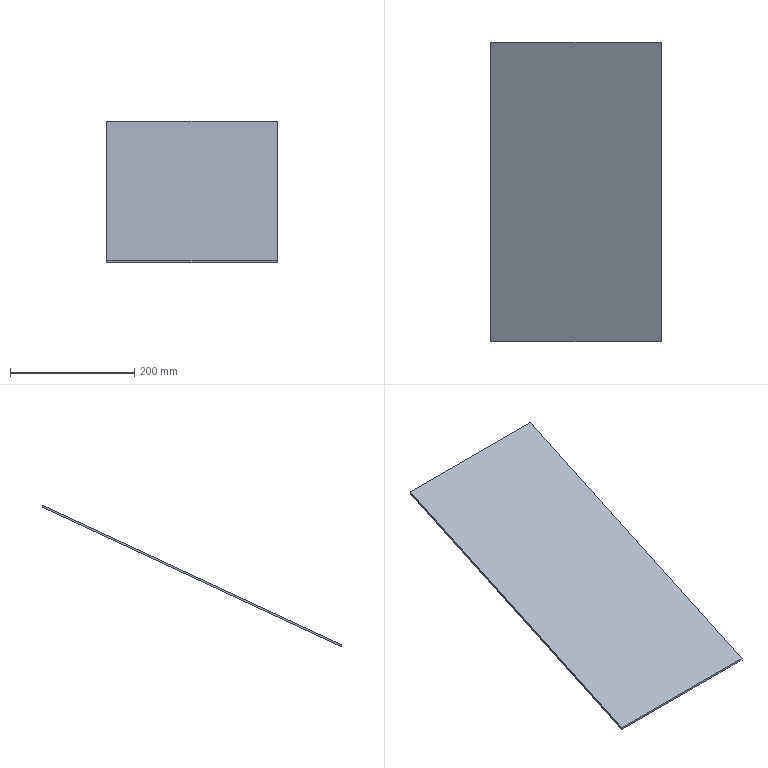Part | NX | features solid 2 | 1 solid | 6 faces | box 274 x 482 x 228.07 mm | volume 437163 mm3 | plane 6
STEP:
#1=CARTESIAN_POINT('',(-137.,22.,-157.195));
#2=VERTEX_POINT('',#1);
#3=CARTESIAN_POINT('',(-137.,22.,-160.505));
#4=VERTEX_POINT('',#3);
#5=CARTESIAN_POINT('',(-137.,22.,-497.5));
#6=DIRECTION('',(0.,0.,-1.));
#7=VECTOR('',#6,1000.);
#8=LINE('',#5,#7);
#9=EDGE_CURVE('',#2,#4,#8,.T.);
#10=ORIENTED_EDGE('',*,*,#9,.T.);
#11=CARTESIAN_POINT('',(-137.,-460.,-385.266));
#12=VERTEX_POINT('',#11);
#13=CARTESIAN_POINT('',(-137.,-98.862,-216.864));
#14=DIRECTION('',(0.,-0.9063,-0.4226));
#15=VECTOR('',#14,1000.);
#16=LINE('',#13,#15);
#17=EDGE_CURVE('',#4,#12,#16,.T.);
#18=ORIENTED_EDGE('',*,*,#17,.T.);
#19=CARTESIAN_POINT('',(-137.,-460.,-381.956));
#20=VERTEX_POINT('',#19);
#21=CARTESIAN_POINT('',(-137.,-460.,-97.5));
#22=DIRECTION('',(0.,0.,1.));
#23=VECTOR('',#22,1000.);
#24=LINE('',#21,#23);
#25=EDGE_CURVE('',#20,#12,#24,.F.);
#26=ORIENTED_EDGE('',*,*,#25,.F.);
#27=CARTESIAN_POINT('',(-137.,-100.13,-214.146));
#28=DIRECTION('',(0.,-0.9063,-0.4226));
#29=VECTOR('',#28,1000.);
#30=LINE('',#27,#29);
#31=EDGE_CURVE('',#2,#20,#30,.T.);
#32=ORIENTED_EDGE('',*,*,#31,.F.);
#33=EDGE_LOOP('',(#10,#18,#26,#32));
#34=FACE_BOUND('',#33,.T.);
#35=CARTESIAN_POINT('',(-137.,32.,-497.5));
#36=DIRECTION('',(1.,0.,0.));
#37=DIRECTION('',(0.,0.,-1.));
#38=AXIS2_PLACEMENT_3D('',#35,#36,#37);
#39=PLANE('',#38);
#40=ADVANCED_FACE('',(#34),#39,.F.);
#41=ORIENTED_EDGE('',*,*,#25,.T.);
#42=CARTESIAN_POINT('',(137.,-460.,-385.266));
#43=VERTEX_POINT('',#42);
#44=CARTESIAN_POINT('',(1125.,-460.,-385.266));
#45=DIRECTION('',(-1.,0.,0.));
#46=VECTOR('',#45,1000.);
#47=LINE('',#44,#46);
#48=EDGE_CURVE('',#12,#43,#47,.F.);
#49=ORIENTED_EDGE('',*,*,#48,.T.);
#50=CARTESIAN_POINT('',(137.,-460.,-381.956));
#51=VERTEX_POINT('',#50);
#52=CARTESIAN_POINT('',(137.,-460.,-497.5));
#53=DIRECTION('',(0.,0.,1.));
#54=VECTOR('',#53,1000.);
#55=LINE('',#52,#54);
#56=EDGE_CURVE('',#51,#43,#55,.F.);
#57=ORIENTED_EDGE('',*,*,#56,.F.);
#58=CARTESIAN_POINT('',(1125.,-460.,-381.956));
#59=DIRECTION('',(-1.,0.,0.));
#60=VECTOR('',#59,1000.);
#61=LINE('',#58,#60);
#62=EDGE_CURVE('',#20,#51,#61,.F.);
#63=ORIENTED_EDGE('',*,*,#62,.F.);
#64=EDGE_LOOP('',(#41,#49,#57,#63));
#65=FACE_BOUND('',#64,.T.);
#66=CARTESIAN_POINT('',(1125.,-460.,-97.5));
#67=DIRECTION('',(0.,-1.,0.));
#68=DIRECTION('',(-1.,0.,0.));
#69=AXIS2_PLACEMENT_3D('',#66,#67,#68);
#70=PLANE('',#69);
#71=ADVANCED_FACE('',(#65),#70,.T.);
#72=ORIENTED_EDGE('',*,*,#56,.T.);
#73=CARTESIAN_POINT('',(137.,22.,-160.505));
#74=VERTEX_POINT('',#73);
#75=CARTESIAN_POINT('',(137.,7.,-167.5));
#76=DIRECTION('',(0.,-0.9063,-0.4226));
#77=VECTOR('',#76,1000.);
#78=LINE('',#75,#77);
#79=EDGE_CURVE('',#74,#43,#78,.T.);
#80=ORIENTED_EDGE('',*,*,#79,.F.);
#81=CARTESIAN_POINT('',(137.,22.,-157.195));
#82=VERTEX_POINT('',#81);
#83=CARTESIAN_POINT('',(137.,22.,26.231));
#84=DIRECTION('',(0.,0.,-1.));
#85=VECTOR('',#84,1000.);
#86=LINE('',#83,#85);
#87=EDGE_CURVE('',#82,#74,#86,.T.);
#88=ORIENTED_EDGE('',*,*,#87,.F.);
#89=CARTESIAN_POINT('',(137.,5.732,-164.781));
#90=DIRECTION('',(0.,-0.9063,-0.4226));
#91=VECTOR('',#90,1000.);
#92=LINE('',#89,#91);
#93=EDGE_CURVE('',#82,#51,#92,.T.);
#94=ORIENTED_EDGE('',*,*,#93,.T.);
#95=EDGE_LOOP('',(#72,#80,#88,#94));
#96=FACE_BOUND('',#95,.T.);
#97=CARTESIAN_POINT('',(137.,32.,-497.5));
#98=DIRECTION('',(-1.,0.,0.));
#99=DIRECTION('',(0.,0.,-1.));
#100=AXIS2_PLACEMENT_3D('',#97,#98,#99);
#101=PLANE('',#100);
#102=ADVANCED_FACE('',(#96),#101,.F.);
#103=CARTESIAN_POINT('',(-17.526,22.,-157.195));
#104=DIRECTION('',(1.,0.,0.));
#105=VECTOR('',#104,1000.);
#106=LINE('',#103,#105);
#107=EDGE_CURVE('',#2,#82,#106,.T.);
#108=ORIENTED_EDGE('',*,*,#107,.T.);
#109=ORIENTED_EDGE('',*,*,#87,.T.);
#110=CARTESIAN_POINT('',(-17.526,22.,-160.505));
#111=DIRECTION('',(1.,0.,0.));
#112=VECTOR('',#111,1000.);
#113=LINE('',#110,#112);
#114=EDGE_CURVE('',#4,#74,#113,.T.);
#115=ORIENTED_EDGE('',*,*,#114,.F.);
#116=ORIENTED_EDGE('',*,*,#9,.F.);
#117=EDGE_LOOP('',(#108,#109,#115,#116));
#118=FACE_BOUND('',#117,.T.);
#119=CARTESIAN_POINT('',(94.724,22.,26.231));
#120=DIRECTION('',(0.,-1.,0.));
#121=DIRECTION('',(0.,0.,-1.));
#122=AXIS2_PLACEMENT_3D('',#119,#120,#121);
#123=PLANE('',#122);
#124=ADVANCED_FACE('',(#118),#123,.F.);
#125=ORIENTED_EDGE('',*,*,#79,.T.);
#126=ORIENTED_EDGE('',*,*,#48,.F.);
#127=ORIENTED_EDGE('',*,*,#17,.F.);
#128=ORIENTED_EDGE('',*,*,#114,.T.);
#129=EDGE_LOOP('',(#125,#126,#127,#128));
#130=FACE_BOUND('',#129,.T.);
#131=CARTESIAN_POINT('',(-17.526,7.,-167.5));
#132=DIRECTION('',(0.,-0.4226,0.9063));
#133=DIRECTION('',(0.,-0.9063,-0.4226));
#134=AXIS2_PLACEMENT_3D('',#131,#132,#133);
#135=PLANE('',#134);
#136=ADVANCED_FACE('',(#130),#135,.F.);
#137=ORIENTED_EDGE('',*,*,#93,.F.);
#138=ORIENTED_EDGE('',*,*,#107,.F.);
#139=ORIENTED_EDGE('',*,*,#31,.T.);
#140=ORIENTED_EDGE('',*,*,#62,.T.);
#141=EDGE_LOOP('',(#137,#138,#139,#140));
#142=FACE_BOUND('',#141,.T.);
#143=CARTESIAN_POINT('',(-17.526,5.732,-164.781));
#144=DIRECTION('',(0.,-0.4226,0.9063));
#145=DIRECTION('',(0.,-0.9063,-0.4226));
#146=AXIS2_PLACEMENT_3D('',#143,#144,#145);
#147=PLANE('',#146);
#148=ADVANCED_FACE('',(#142),#147,.T.);
#149=CLOSED_SHELL('',(#40,#71,#102,#124,#136,#148));
#150=MANIFOLD_SOLID_BREP('',#149);
#151=(LENGTH_UNIT()NAMED_UNIT(*)SI_UNIT(.MILLI.,.METRE.));
#152=UNCERTAINTY_MEASURE_WITH_UNIT(LENGTH_MEASURE(0.00001),#151,'','');
#153=(NAMED_UNIT(*)PLANE_ANGLE_UNIT()SI_UNIT($,.RADIAN.));
#154=(NAMED_UNIT(*)SI_UNIT($,.STERADIAN.)SOLID_ANGLE_UNIT());
#155=(GEOMETRIC_REPRESENTATION_CONTEXT(3)GLOBAL_UNCERTAINTY_ASSIGNED_CONTEXT((#152))GLOBAL_UNIT_ASSIGNED_CONTEXT((#151,#153,#154))REPRESENTATION_CONTEXT('',''));
#156=ADVANCED_BREP_SHAPE_REPRESENTATION('',(#150),#155);